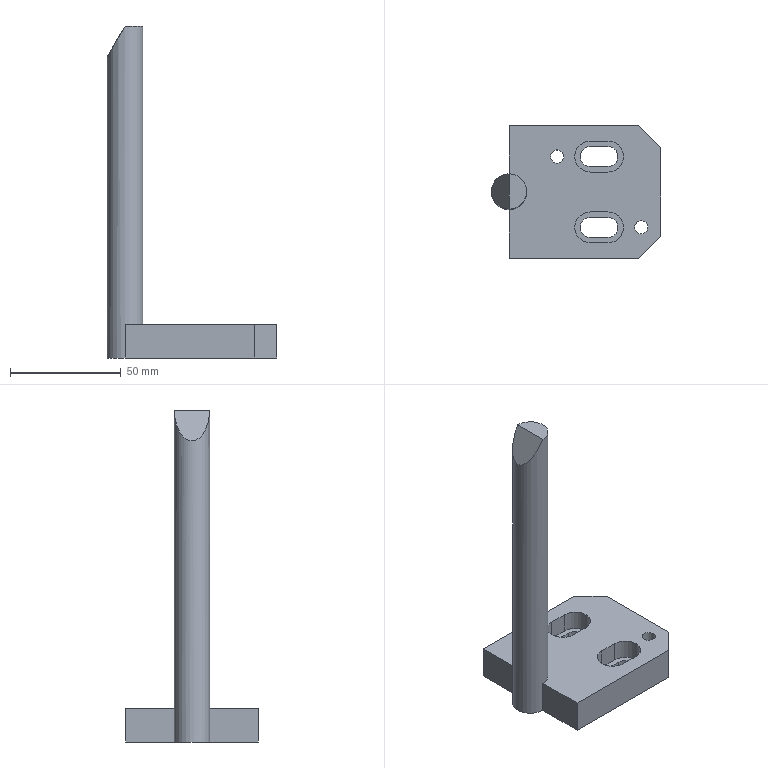Part | NX | features solid 2 | 1 solid | 32 faces | box 76.5 x 60 x 150 mm | volume 80948 mm3 | plane 21 | cylinder 11 | commonest cylinder face diameters 9 x4 14 x4 6 x2 16 x1
STEP:
#1=CARTESIAN_POINT('',(676.5,-352.,-140.));
#2=VERTEX_POINT('',#1);
#3=CARTESIAN_POINT('',(676.5,-352.,-125.));
#4=VERTEX_POINT('',#3);
#5=CARTESIAN_POINT('',(676.5,-352.,-140.));
#6=DIRECTION('',(0.,0.,1.));
#7=VECTOR('',#6,1000.);
#8=LINE('',#5,#7);
#9=EDGE_CURVE('',#2,#4,#8,.T.);
#10=ORIENTED_EDGE('',*,*,#9,.F.);
#11=CARTESIAN_POINT('',(676.5,-368.,-140.));
#12=VERTEX_POINT('',#11);
#13=CARTESIAN_POINT('',(676.5,-360.,-140.));
#14=DIRECTION('',(0.,0.,1.));
#15=DIRECTION('',(0.,1.,0.));
#16=AXIS2_PLACEMENT_3D('',#13,#14,#15);
#17=CIRCLE('',#16,8.);
#18=EDGE_CURVE('',#2,#12,#17,.T.);
#19=ORIENTED_EDGE('',*,*,#18,.T.);
#20=CARTESIAN_POINT('',(676.5,-368.,-125.));
#21=VERTEX_POINT('',#20);
#22=CARTESIAN_POINT('',(676.5,-368.,-140.));
#23=DIRECTION('',(0.,0.,1.));
#24=VECTOR('',#23,1000.);
#25=LINE('',#22,#24);
#26=EDGE_CURVE('',#21,#12,#25,.F.);
#27=ORIENTED_EDGE('',*,*,#26,.F.);
#28=CARTESIAN_POINT('',(676.5,-360.,-125.));
#29=DIRECTION('',(0.,0.,1.));
#30=DIRECTION('',(-1.,0.,0.));
#31=AXIS2_PLACEMENT_3D('',#28,#29,#30);
#32=CIRCLE('',#31,8.);
#33=EDGE_CURVE('',#21,#4,#32,.T.);
#34=ORIENTED_EDGE('',*,*,#33,.T.);
#35=EDGE_LOOP('',(#10,#19,#27,#34));
#36=FACE_BOUND('',#35,.T.);
#37=CARTESIAN_POINT('',(676.5,-368.,10.));
#38=VERTEX_POINT('',#37);
#39=CARTESIAN_POINT('',(676.5,-352.,10.));
#40=VERTEX_POINT('',#39);
#41=CARTESIAN_POINT('',(676.5,-360.,10.));
#42=DIRECTION('',(0.,0.,-1.));
#43=DIRECTION('',(-1.,0.,0.));
#44=AXIS2_PLACEMENT_3D('',#41,#42,#43);
#45=CIRCLE('',#44,8.);
#46=EDGE_CURVE('',#38,#40,#45,.F.);
#47=ORIENTED_EDGE('',*,*,#46,.F.);
#48=CARTESIAN_POINT('',(676.5,-360.,10.));
#49=DIRECTION('',(0.866,0.,-0.5));
#50=DIRECTION('',(0.5,0.,0.866));
#51=AXIS2_PLACEMENT_3D('',#48,#49,#50);
#52=ELLIPSE('',#51,16.,8.);
#53=EDGE_CURVE('',#40,#38,#52,.F.);
#54=ORIENTED_EDGE('',*,*,#53,.F.);
#55=EDGE_LOOP('',(#47,#54));
#56=FACE_BOUND('',#55,.T.);
#57=CARTESIAN_POINT('',(676.5,-360.,-140.));
#58=DIRECTION('',(0.,0.,1.));
#59=DIRECTION('',(-1.,0.,0.));
#60=AXIS2_PLACEMENT_3D('',#57,#58,#59);
#61=CYLINDRICAL_SURFACE('',#60,8.);
#62=ADVANCED_FACE('',(#36,#56),#61,.T.);
#63=ORIENTED_EDGE('',*,*,#46,.T.);
#64=CARTESIAN_POINT('',(676.5,-360.,10.));
#65=DIRECTION('',(0.,1.,0.));
#66=VECTOR('',#65,1000.);
#67=LINE('',#64,#66);
#68=EDGE_CURVE('',#38,#40,#67,.T.);
#69=ORIENTED_EDGE('',*,*,#68,.F.);
#70=EDGE_LOOP('',(#63,#69));
#71=FACE_BOUND('',#70,.T.);
#72=CARTESIAN_POINT('',(682.,-360.,10.));
#73=DIRECTION('',(0.,0.,1.));
#74=DIRECTION('',(-1.,0.,0.));
#75=AXIS2_PLACEMENT_3D('',#72,#73,#74);
#76=PLANE('',#75);
#77=ADVANCED_FACE('',(#71),#76,.T.);
#78=CARTESIAN_POINT('',(695.2,-344.,-125.));
#79=VERTEX_POINT('',#78);
#80=CARTESIAN_POINT('',(698.2,-344.,-125.));
#81=DIRECTION('',(0.,0.,1.));
#82=DIRECTION('',(-1.,0.,0.));
#83=AXIS2_PLACEMENT_3D('',#80,#81,#82);
#84=CIRCLE('',#83,3.);
#85=EDGE_CURVE('',#79,#79,#84,.F.);
#86=ORIENTED_EDGE('',*,*,#85,.T.);
#87=EDGE_LOOP('',(#86));
#88=FACE_BOUND('',#87,.T.);
#89=CARTESIAN_POINT('',(713.2,-351.,-125.));
#90=VERTEX_POINT('',#89);
#91=CARTESIAN_POINT('',(713.2,-337.,-125.));
#92=VERTEX_POINT('',#91);
#93=CARTESIAN_POINT('',(713.2,-344.,-125.));
#94=DIRECTION('',(0.,0.,1.));
#95=DIRECTION('',(-1.,0.,0.));
#96=AXIS2_PLACEMENT_3D('',#93,#94,#95);
#97=CIRCLE('',#96,7.);
#98=EDGE_CURVE('',#90,#92,#97,.F.);
#99=ORIENTED_EDGE('',*,*,#98,.T.);
#100=CARTESIAN_POINT('',(721.2,-337.,-125.));
#101=VERTEX_POINT('',#100);
#102=CARTESIAN_POINT('',(768.,-337.,-125.));
#103=DIRECTION('',(1.,0.,0.));
#104=VECTOR('',#103,1000.);
#105=LINE('',#102,#104);
#106=EDGE_CURVE('',#92,#101,#105,.T.);
#107=ORIENTED_EDGE('',*,*,#106,.T.);
#108=CARTESIAN_POINT('',(721.2,-351.,-125.));
#109=VERTEX_POINT('',#108);
#110=CARTESIAN_POINT('',(721.2,-344.,-125.));
#111=DIRECTION('',(0.,0.,1.));
#112=DIRECTION('',(-1.,0.,0.));
#113=AXIS2_PLACEMENT_3D('',#110,#111,#112);
#114=CIRCLE('',#113,7.);
#115=EDGE_CURVE('',#101,#109,#114,.F.);
#116=ORIENTED_EDGE('',*,*,#115,.T.);
#117=CARTESIAN_POINT('',(768.,-351.,-125.));
#118=DIRECTION('',(1.,0.,0.));
#119=VECTOR('',#118,1000.);
#120=LINE('',#117,#119);
#121=EDGE_CURVE('',#90,#109,#120,.T.);
#122=ORIENTED_EDGE('',*,*,#121,.F.);
#123=EDGE_LOOP('',(#99,#107,#116,#122));
#124=FACE_BOUND('',#123,.T.);
#125=CARTESIAN_POINT('',(733.2,-376.,-125.));
#126=VERTEX_POINT('',#125);
#127=CARTESIAN_POINT('',(736.2,-376.,-125.));
#128=DIRECTION('',(0.,0.,1.));
#129=DIRECTION('',(-1.,0.,0.));
#130=AXIS2_PLACEMENT_3D('',#127,#128,#129);
#131=CIRCLE('',#130,3.);
#132=EDGE_CURVE('',#126,#126,#131,.F.);
#133=ORIENTED_EDGE('',*,*,#132,.T.);
#134=EDGE_LOOP('',(#133));
#135=FACE_BOUND('',#134,.T.);
#136=CARTESIAN_POINT('',(713.2,-383.,-125.));
#137=VERTEX_POINT('',#136);
#138=CARTESIAN_POINT('',(721.2,-383.,-125.));
#139=VERTEX_POINT('',#138);
#140=CARTESIAN_POINT('',(713.2,-383.,-125.));
#141=DIRECTION('',(1.,0.,0.));
#142=VECTOR('',#141,1000.);
#143=LINE('',#140,#142);
#144=EDGE_CURVE('',#137,#139,#143,.T.);
#145=ORIENTED_EDGE('',*,*,#144,.F.);
#146=CARTESIAN_POINT('',(713.2,-369.,-125.));
#147=VERTEX_POINT('',#146);
#148=CARTESIAN_POINT('',(713.2,-376.,-125.));
#149=DIRECTION('',(0.,0.,1.));
#150=DIRECTION('',(-1.,0.,0.));
#151=AXIS2_PLACEMENT_3D('',#148,#149,#150);
#152=CIRCLE('',#151,7.);
#153=EDGE_CURVE('',#147,#137,#152,.T.);
#154=ORIENTED_EDGE('',*,*,#153,.F.);
#155=CARTESIAN_POINT('',(721.2,-369.,-125.));
#156=VERTEX_POINT('',#155);
#157=CARTESIAN_POINT('',(713.2,-369.,-125.));
#158=DIRECTION('',(1.,0.,0.));
#159=VECTOR('',#158,1000.);
#160=LINE('',#157,#159);
#161=EDGE_CURVE('',#147,#156,#160,.T.);
#162=ORIENTED_EDGE('',*,*,#161,.T.);
#163=CARTESIAN_POINT('',(721.2,-376.,-125.));
#164=DIRECTION('',(0.,0.,1.));
#165=DIRECTION('',(-1.,0.,0.));
#166=AXIS2_PLACEMENT_3D('',#163,#164,#165);
#167=CIRCLE('',#166,7.);
#168=EDGE_CURVE('',#139,#156,#167,.T.);
#169=ORIENTED_EDGE('',*,*,#168,.F.);
#170=EDGE_LOOP('',(#145,#154,#162,#169));
#171=FACE_BOUND('',#170,.T.);
#172=CARTESIAN_POINT('',(676.5,-390.,-125.));
#173=VERTEX_POINT('',#172);
#174=CARTESIAN_POINT('',(735.,-390.,-125.));
#175=VERTEX_POINT('',#174);
#176=CARTESIAN_POINT('',(688.,-390.,-125.));
#177=DIRECTION('',(1.,0.,0.));
#178=VECTOR('',#177,1000.);
#179=LINE('',#176,#178);
#180=EDGE_CURVE('',#173,#175,#179,.T.);
#181=ORIENTED_EDGE('',*,*,#180,.T.);
#182=CARTESIAN_POINT('',(745.,-380.,-125.));
#183=VERTEX_POINT('',#182);
#184=CARTESIAN_POINT('',(766.5,-358.5,-125.));
#185=DIRECTION('',(-0.7071,-0.7071,0.));
#186=VECTOR('',#185,1000.);
#187=LINE('',#184,#186);
#188=EDGE_CURVE('',#175,#183,#187,.F.);
#189=ORIENTED_EDGE('',*,*,#188,.T.);
#190=CARTESIAN_POINT('',(745.,-340.,-125.));
#191=VERTEX_POINT('',#190);
#192=CARTESIAN_POINT('',(745.,-360.,-125.));
#193=DIRECTION('',(0.,-1.,0.));
#194=VECTOR('',#193,1000.);
#195=LINE('',#192,#194);
#196=EDGE_CURVE('',#183,#191,#195,.F.);
#197=ORIENTED_EDGE('',*,*,#196,.T.);
#198=CARTESIAN_POINT('',(735.,-330.,-125.));
#199=VERTEX_POINT('',#198);
#200=CARTESIAN_POINT('',(766.5,-361.5,-125.));
#201=DIRECTION('',(-0.7071,0.7071,0.));
#202=VECTOR('',#201,1000.);
#203=LINE('',#200,#202);
#204=EDGE_CURVE('',#191,#199,#203,.T.);
#205=ORIENTED_EDGE('',*,*,#204,.T.);
#206=CARTESIAN_POINT('',(676.5,-330.,-125.));
#207=VERTEX_POINT('',#206);
#208=CARTESIAN_POINT('',(688.,-330.,-125.));
#209=DIRECTION('',(1.,0.,0.));
#210=VECTOR('',#209,1000.);
#211=LINE('',#208,#210);
#212=EDGE_CURVE('',#207,#199,#211,.T.);
#213=ORIENTED_EDGE('',*,*,#212,.F.);
#214=CARTESIAN_POINT('',(676.5,-330.,-125.));
#215=DIRECTION('',(0.,-1.,0.));
#216=VECTOR('',#215,1000.);
#217=LINE('',#214,#216);
#218=EDGE_CURVE('',#207,#4,#217,.T.);
#219=ORIENTED_EDGE('',*,*,#218,.T.);
#220=ORIENTED_EDGE('',*,*,#33,.F.);
#221=CARTESIAN_POINT('',(676.5,-330.,-125.));
#222=DIRECTION('',(0.,-1.,0.));
#223=VECTOR('',#222,1000.);
#224=LINE('',#221,#223);
#225=EDGE_CURVE('',#21,#173,#224,.T.);
#226=ORIENTED_EDGE('',*,*,#225,.T.);
#227=EDGE_LOOP('',(#181,#189,#197,#205,#213,#219,#220,#226));
#228=FACE_BOUND('',#227,.T.);
#229=CARTESIAN_POINT('',(768.,-360.,-125.));
#230=DIRECTION('',(0.,0.,1.));
#231=DIRECTION('',(-1.,0.,0.));
#232=AXIS2_PLACEMENT_3D('',#229,#230,#231);
#233=PLANE('',#232);
#234=ADVANCED_FACE('',(#88,#124,#135,#171,#228),#233,.T.);
#235=CARTESIAN_POINT('',(695.2,-344.,-140.));
#236=VERTEX_POINT('',#235);
#237=CARTESIAN_POINT('',(698.2,-344.,-140.));
#238=DIRECTION('',(0.,0.,1.));
#239=DIRECTION('',(-1.,0.,0.));
#240=AXIS2_PLACEMENT_3D('',#237,#238,#239);
#241=CIRCLE('',#240,3.);
#242=EDGE_CURVE('',#236,#236,#241,.T.);
#243=ORIENTED_EDGE('',*,*,#242,.T.);
#244=EDGE_LOOP('',(#243));
#245=FACE_BOUND('',#244,.T.);
#246=CARTESIAN_POINT('',(721.2,-380.5,-140.));
#247=VERTEX_POINT('',#246);
#248=CARTESIAN_POINT('',(721.2,-371.5,-140.));
#249=VERTEX_POINT('',#248);
#250=CARTESIAN_POINT('',(721.2,-376.,-140.));
#251=DIRECTION('',(0.,0.,1.));
#252=DIRECTION('',(-1.,0.,0.));
#253=AXIS2_PLACEMENT_3D('',#250,#251,#252);
#254=CIRCLE('',#253,4.5);
#255=EDGE_CURVE('',#247,#249,#254,.T.);
#256=ORIENTED_EDGE('',*,*,#255,.T.);
#257=CARTESIAN_POINT('',(713.2,-371.5,-140.));
#258=VERTEX_POINT('',#257);
#259=CARTESIAN_POINT('',(713.2,-371.5,-140.));
#260=DIRECTION('',(1.,0.,0.));
#261=VECTOR('',#260,1000.);
#262=LINE('',#259,#261);
#263=EDGE_CURVE('',#258,#249,#262,.T.);
#264=ORIENTED_EDGE('',*,*,#263,.F.);
#265=CARTESIAN_POINT('',(713.2,-380.5,-140.));
#266=VERTEX_POINT('',#265);
#267=CARTESIAN_POINT('',(713.2,-376.,-140.));
#268=DIRECTION('',(0.,0.,1.));
#269=DIRECTION('',(-1.,0.,0.));
#270=AXIS2_PLACEMENT_3D('',#267,#268,#269);
#271=CIRCLE('',#270,4.5);
#272=EDGE_CURVE('',#258,#266,#271,.T.);
#273=ORIENTED_EDGE('',*,*,#272,.T.);
#274=CARTESIAN_POINT('',(713.2,-380.5,-140.));
#275=DIRECTION('',(1.,0.,0.));
#276=VECTOR('',#275,1000.);
#277=LINE('',#274,#276);
#278=EDGE_CURVE('',#266,#247,#277,.T.);
#279=ORIENTED_EDGE('',*,*,#278,.T.);
#280=EDGE_LOOP('',(#256,#264,#273,#279));
#281=FACE_BOUND('',#280,.T.);
#282=CARTESIAN_POINT('',(733.2,-376.,-140.));
#283=VERTEX_POINT('',#282);
#284=CARTESIAN_POINT('',(736.2,-376.,-140.));
#285=DIRECTION('',(0.,0.,1.));
#286=DIRECTION('',(-1.,0.,0.));
#287=AXIS2_PLACEMENT_3D('',#284,#285,#286);
#288=CIRCLE('',#287,3.);
#289=EDGE_CURVE('',#283,#283,#288,.T.);
#290=ORIENTED_EDGE('',*,*,#289,.T.);
#291=EDGE_LOOP('',(#290));
#292=FACE_BOUND('',#291,.T.);
#293=CARTESIAN_POINT('',(721.2,-348.5,-140.));
#294=VERTEX_POINT('',#293);
#295=CARTESIAN_POINT('',(721.2,-339.5,-140.));
#296=VERTEX_POINT('',#295);
#297=CARTESIAN_POINT('',(721.2,-344.,-140.));
#298=DIRECTION('',(0.,0.,1.));
#299=DIRECTION('',(-1.,0.,0.));
#300=AXIS2_PLACEMENT_3D('',#297,#298,#299);
#301=CIRCLE('',#300,4.5);
#302=EDGE_CURVE('',#294,#296,#301,.T.);
#303=ORIENTED_EDGE('',*,*,#302,.T.);
#304=CARTESIAN_POINT('',(713.2,-339.5,-140.));
#305=VERTEX_POINT('',#304);
#306=CARTESIAN_POINT('',(723.2,-339.5,-140.));
#307=DIRECTION('',(-1.,0.,0.));
#308=VECTOR('',#307,1000.);
#309=LINE('',#306,#308);
#310=EDGE_CURVE('',#296,#305,#309,.T.);
#311=ORIENTED_EDGE('',*,*,#310,.T.);
#312=CARTESIAN_POINT('',(713.2,-348.5,-140.));
#313=VERTEX_POINT('',#312);
#314=CARTESIAN_POINT('',(713.2,-344.,-140.));
#315=DIRECTION('',(0.,0.,1.));
#316=DIRECTION('',(-1.,0.,0.));
#317=AXIS2_PLACEMENT_3D('',#314,#315,#316);
#318=CIRCLE('',#317,4.5);
#319=EDGE_CURVE('',#305,#313,#318,.T.);
#320=ORIENTED_EDGE('',*,*,#319,.T.);
#321=CARTESIAN_POINT('',(723.2,-348.5,-140.));
#322=DIRECTION('',(-1.,0.,0.));
#323=VECTOR('',#322,1000.);
#324=LINE('',#321,#323);
#325=EDGE_CURVE('',#294,#313,#324,.T.);
#326=ORIENTED_EDGE('',*,*,#325,.F.);
#327=EDGE_LOOP('',(#303,#311,#320,#326));
#328=FACE_BOUND('',#327,.T.);
#329=CARTESIAN_POINT('',(745.,-340.,-140.));
#330=VERTEX_POINT('',#329);
#331=CARTESIAN_POINT('',(745.,-380.,-140.));
#332=VERTEX_POINT('',#331);
#333=CARTESIAN_POINT('',(745.,-320.,-140.));
#334=DIRECTION('',(0.,1.,0.));
#335=VECTOR('',#334,1000.);
#336=LINE('',#333,#335);
#337=EDGE_CURVE('',#330,#332,#336,.F.);
#338=ORIENTED_EDGE('',*,*,#337,.T.);
#339=CARTESIAN_POINT('',(735.,-390.,-140.));
#340=VERTEX_POINT('',#339);
#341=CARTESIAN_POINT('',(745.,-380.,-140.));
#342=DIRECTION('',(0.7071,0.7071,0.));
#343=VECTOR('',#342,1000.);
#344=LINE('',#341,#343);
#345=EDGE_CURVE('',#332,#340,#344,.F.);
#346=ORIENTED_EDGE('',*,*,#345,.T.);
#347=CARTESIAN_POINT('',(676.5,-390.,-140.));
#348=VERTEX_POINT('',#347);
#349=CARTESIAN_POINT('',(688.,-390.,-140.));
#350=DIRECTION('',(1.,0.,0.));
#351=VECTOR('',#350,1000.);
#352=LINE('',#349,#351);
#353=EDGE_CURVE('',#348,#340,#352,.T.);
#354=ORIENTED_EDGE('',*,*,#353,.F.);
#355=CARTESIAN_POINT('',(676.5,-330.,-140.));
#356=DIRECTION('',(0.,-1.,0.));
#357=VECTOR('',#356,1000.);
#358=LINE('',#355,#357);
#359=EDGE_CURVE('',#12,#348,#358,.T.);
#360=ORIENTED_EDGE('',*,*,#359,.F.);
#361=ORIENTED_EDGE('',*,*,#18,.F.);
#362=CARTESIAN_POINT('',(676.5,-330.,-140.));
#363=VERTEX_POINT('',#362);
#364=CARTESIAN_POINT('',(676.5,-330.,-140.));
#365=DIRECTION('',(0.,-1.,0.));
#366=VECTOR('',#365,1000.);
#367=LINE('',#364,#366);
#368=EDGE_CURVE('',#363,#2,#367,.T.);
#369=ORIENTED_EDGE('',*,*,#368,.F.);
#370=CARTESIAN_POINT('',(735.,-330.,-140.));
#371=VERTEX_POINT('',#370);
#372=CARTESIAN_POINT('',(688.,-330.,-140.));
#373=DIRECTION('',(1.,0.,0.));
#374=VECTOR('',#373,1000.);
#375=LINE('',#372,#374);
#376=EDGE_CURVE('',#363,#371,#375,.T.);
#377=ORIENTED_EDGE('',*,*,#376,.T.);
#378=CARTESIAN_POINT('',(735.,-330.,-140.));
#379=DIRECTION('',(0.7071,-0.7071,0.));
#380=VECTOR('',#379,1000.);
#381=LINE('',#378,#380);
#382=EDGE_CURVE('',#371,#330,#381,.T.);
#383=ORIENTED_EDGE('',*,*,#382,.T.);
#384=EDGE_LOOP('',(#338,#346,#354,#360,#361,#369,#377,#383));
#385=FACE_BOUND('',#384,.T.);
#386=CARTESIAN_POINT('',(768.,-360.,-140.));
#387=DIRECTION('',(0.,0.,1.));
#388=DIRECTION('',(-1.,0.,0.));
#389=AXIS2_PLACEMENT_3D('',#386,#387,#388);
#390=PLANE('',#389);
#391=ADVANCED_FACE('',(#245,#281,#292,#328,#385),#390,.F.);
#392=ORIENTED_EDGE('',*,*,#212,.T.);
#393=CARTESIAN_POINT('',(735.,-330.,-125.));
#394=DIRECTION('',(0.,0.,-1.));
#395=VECTOR('',#394,1000.);
#396=LINE('',#393,#395);
#397=EDGE_CURVE('',#199,#371,#396,.T.);
#398=ORIENTED_EDGE('',*,*,#397,.T.);
#399=ORIENTED_EDGE('',*,*,#376,.F.);
#400=CARTESIAN_POINT('',(676.5,-330.,-125.));
#401=DIRECTION('',(0.,0.,-1.));
#402=VECTOR('',#401,1000.);
#403=LINE('',#400,#402);
#404=EDGE_CURVE('',#207,#363,#403,.T.);
#405=ORIENTED_EDGE('',*,*,#404,.F.);
#406=EDGE_LOOP('',(#392,#398,#399,#405));
#407=FACE_BOUND('',#406,.T.);
#408=CARTESIAN_POINT('',(688.,-330.,-125.));
#409=DIRECTION('',(0.,1.,0.));
#410=DIRECTION('',(0.,0.,-1.));
#411=AXIS2_PLACEMENT_3D('',#408,#409,#410);
#412=PLANE('',#411);
#413=ADVANCED_FACE('',(#407),#412,.T.);
#414=ORIENTED_EDGE('',*,*,#353,.T.);
#415=CARTESIAN_POINT('',(735.,-390.,-125.));
#416=DIRECTION('',(0.,0.,1.));
#417=VECTOR('',#416,1000.);
#418=LINE('',#415,#417);
#419=EDGE_CURVE('',#340,#175,#418,.T.);
#420=ORIENTED_EDGE('',*,*,#419,.T.);
#421=ORIENTED_EDGE('',*,*,#180,.F.);
#422=CARTESIAN_POINT('',(676.5,-390.,-125.));
#423=DIRECTION('',(0.,0.,-1.));
#424=VECTOR('',#423,1000.);
#425=LINE('',#422,#424);
#426=EDGE_CURVE('',#173,#348,#425,.T.);
#427=ORIENTED_EDGE('',*,*,#426,.T.);
#428=EDGE_LOOP('',(#414,#420,#421,#427));
#429=FACE_BOUND('',#428,.T.);
#430=CARTESIAN_POINT('',(688.,-390.,-125.));
#431=DIRECTION('',(0.,1.,0.));
#432=DIRECTION('',(-1.,0.,0.));
#433=AXIS2_PLACEMENT_3D('',#430,#431,#432);
#434=PLANE('',#433);
#435=ADVANCED_FACE('',(#429),#434,.F.);
#436=ORIENTED_EDGE('',*,*,#368,.T.);
#437=ORIENTED_EDGE('',*,*,#9,.T.);
#438=ORIENTED_EDGE('',*,*,#218,.F.);
#439=ORIENTED_EDGE('',*,*,#404,.T.);
#440=EDGE_LOOP('',(#436,#437,#438,#439));
#441=FACE_BOUND('',#440,.T.);
#442=CARTESIAN_POINT('',(676.5,-330.,-125.));
#443=DIRECTION('',(1.,0.,0.));
#444=DIRECTION('',(0.,0.,1.));
#445=AXIS2_PLACEMENT_3D('',#442,#443,#444);
#446=PLANE('',#445);
#447=ADVANCED_FACE('',(#441),#446,.F.);
#448=CARTESIAN_POINT('',(713.2,-371.5,-134.));
#449=VERTEX_POINT('',#448);
#450=CARTESIAN_POINT('',(721.2,-371.5,-134.));
#451=VERTEX_POINT('',#450);
#452=CARTESIAN_POINT('',(713.2,-371.5,-134.));
#453=DIRECTION('',(1.,0.,0.));
#454=VECTOR('',#453,1000.);
#455=LINE('',#452,#454);
#456=EDGE_CURVE('',#449,#451,#455,.T.);
#457=ORIENTED_EDGE('',*,*,#456,.F.);
#458=CARTESIAN_POINT('',(713.2,-371.5,-124.));
#459=DIRECTION('',(0.,0.,-1.));
#460=VECTOR('',#459,1000.);
#461=LINE('',#458,#460);
#462=EDGE_CURVE('',#449,#258,#461,.T.);
#463=ORIENTED_EDGE('',*,*,#462,.T.);
#464=ORIENTED_EDGE('',*,*,#263,.T.);
#465=CARTESIAN_POINT('',(721.2,-371.5,-124.));
#466=DIRECTION('',(0.,0.,-1.));
#467=VECTOR('',#466,1000.);
#468=LINE('',#465,#467);
#469=EDGE_CURVE('',#451,#249,#468,.T.);
#470=ORIENTED_EDGE('',*,*,#469,.F.);
#471=EDGE_LOOP('',(#457,#463,#464,#470));
#472=FACE_BOUND('',#471,.T.);
#473=CARTESIAN_POINT('',(713.2,-371.5,-124.));
#474=DIRECTION('',(0.,1.,0.));
#475=DIRECTION('',(0.,0.,-1.));
#476=AXIS2_PLACEMENT_3D('',#473,#474,#475);
#477=PLANE('',#476);
#478=ADVANCED_FACE('',(#472),#477,.F.);
#479=ORIENTED_EDGE('',*,*,#462,.F.);
#480=CARTESIAN_POINT('',(713.2,-380.5,-134.));
#481=VERTEX_POINT('',#480);
#482=CARTESIAN_POINT('',(713.2,-376.,-134.));
#483=DIRECTION('',(0.,0.,1.));
#484=DIRECTION('',(-1.,0.,0.));
#485=AXIS2_PLACEMENT_3D('',#482,#483,#484);
#486=CIRCLE('',#485,4.5);
#487=EDGE_CURVE('',#449,#481,#486,.T.);
#488=ORIENTED_EDGE('',*,*,#487,.T.);
#489=CARTESIAN_POINT('',(713.2,-380.5,-124.));
#490=DIRECTION('',(0.,0.,-1.));
#491=VECTOR('',#490,1000.);
#492=LINE('',#489,#491);
#493=EDGE_CURVE('',#481,#266,#492,.T.);
#494=ORIENTED_EDGE('',*,*,#493,.T.);
#495=ORIENTED_EDGE('',*,*,#272,.F.);
#496=EDGE_LOOP('',(#479,#488,#494,#495));
#497=FACE_BOUND('',#496,.T.);
#498=CARTESIAN_POINT('',(713.2,-376.,-124.));
#499=DIRECTION('',(0.,0.,-1.));
#500=DIRECTION('',(1.,0.,0.));
#501=AXIS2_PLACEMENT_3D('',#498,#499,#500);
#502=CYLINDRICAL_SURFACE('',#501,4.5);
#503=ADVANCED_FACE('',(#497),#502,.F.);
#504=ORIENTED_EDGE('',*,*,#493,.F.);
#505=CARTESIAN_POINT('',(721.2,-380.5,-134.));
#506=VERTEX_POINT('',#505);
#507=CARTESIAN_POINT('',(713.2,-380.5,-134.));
#508=DIRECTION('',(1.,0.,0.));
#509=VECTOR('',#508,1000.);
#510=LINE('',#507,#509);
#511=EDGE_CURVE('',#481,#506,#510,.T.);
#512=ORIENTED_EDGE('',*,*,#511,.T.);
#513=CARTESIAN_POINT('',(721.2,-380.5,-124.));
#514=DIRECTION('',(0.,0.,-1.));
#515=VECTOR('',#514,1000.);
#516=LINE('',#513,#515);
#517=EDGE_CURVE('',#506,#247,#516,.T.);
#518=ORIENTED_EDGE('',*,*,#517,.T.);
#519=ORIENTED_EDGE('',*,*,#278,.F.);
#520=EDGE_LOOP('',(#504,#512,#518,#519));
#521=FACE_BOUND('',#520,.T.);
#522=CARTESIAN_POINT('',(713.2,-380.5,-124.));
#523=DIRECTION('',(0.,1.,0.));
#524=DIRECTION('',(0.,0.,-1.));
#525=AXIS2_PLACEMENT_3D('',#522,#523,#524);
#526=PLANE('',#525);
#527=ADVANCED_FACE('',(#521),#526,.T.);
#528=ORIENTED_EDGE('',*,*,#517,.F.);
#529=CARTESIAN_POINT('',(721.2,-376.,-134.));
#530=DIRECTION('',(0.,0.,1.));
#531=DIRECTION('',(-1.,0.,0.));
#532=AXIS2_PLACEMENT_3D('',#529,#530,#531);
#533=CIRCLE('',#532,4.5);
#534=EDGE_CURVE('',#506,#451,#533,.T.);
#535=ORIENTED_EDGE('',*,*,#534,.T.);
#536=ORIENTED_EDGE('',*,*,#469,.T.);
#537=ORIENTED_EDGE('',*,*,#255,.F.);
#538=EDGE_LOOP('',(#528,#535,#536,#537));
#539=FACE_BOUND('',#538,.T.);
#540=CARTESIAN_POINT('',(721.2,-376.,-124.));
#541=DIRECTION('',(0.,0.,-1.));
#542=DIRECTION('',(1.,0.,0.));
#543=AXIS2_PLACEMENT_3D('',#540,#541,#542);
#544=CYLINDRICAL_SURFACE('',#543,4.5);
#545=ADVANCED_FACE('',(#539),#544,.F.);
#546=ORIENTED_EDGE('',*,*,#225,.F.);
#547=ORIENTED_EDGE('',*,*,#26,.T.);
#548=ORIENTED_EDGE('',*,*,#359,.T.);
#549=ORIENTED_EDGE('',*,*,#426,.F.);
#550=EDGE_LOOP('',(#546,#547,#548,#549));
#551=FACE_BOUND('',#550,.T.);
#552=CARTESIAN_POINT('',(676.5,-330.,-125.));
#553=DIRECTION('',(1.,0.,0.));
#554=DIRECTION('',(0.,0.,1.));
#555=AXIS2_PLACEMENT_3D('',#552,#553,#554);
#556=PLANE('',#555);
#557=ADVANCED_FACE('',(#551),#556,.F.);
#558=CARTESIAN_POINT('',(713.2,-337.,-134.));
#559=VERTEX_POINT('',#558);
#560=CARTESIAN_POINT('',(713.2,-337.,-124.));
#561=DIRECTION('',(0.,0.,-1.));
#562=VECTOR('',#561,1000.);
#563=LINE('',#560,#562);
#564=EDGE_CURVE('',#92,#559,#563,.T.);
#565=ORIENTED_EDGE('',*,*,#564,.T.);
#566=CARTESIAN_POINT('',(721.2,-337.,-134.));
#567=VERTEX_POINT('',#566);
#568=CARTESIAN_POINT('',(723.2,-337.,-134.));
#569=DIRECTION('',(-1.,0.,0.));
#570=VECTOR('',#569,1000.);
#571=LINE('',#568,#570);
#572=EDGE_CURVE('',#567,#559,#571,.T.);
#573=ORIENTED_EDGE('',*,*,#572,.F.);
#574=CARTESIAN_POINT('',(721.2,-337.,-124.));
#575=DIRECTION('',(0.,0.,-1.));
#576=VECTOR('',#575,1000.);
#577=LINE('',#574,#576);
#578=EDGE_CURVE('',#101,#567,#577,.T.);
#579=ORIENTED_EDGE('',*,*,#578,.F.);
#580=ORIENTED_EDGE('',*,*,#106,.F.);
#581=EDGE_LOOP('',(#565,#573,#579,#580));
#582=FACE_BOUND('',#581,.T.);
#583=CARTESIAN_POINT('',(723.2,-337.,-124.));
#584=DIRECTION('',(0.,-1.,0.));
#585=DIRECTION('',(0.,0.,1.));
#586=AXIS2_PLACEMENT_3D('',#583,#584,#585);
#587=PLANE('',#586);
#588=ADVANCED_FACE('',(#582),#587,.T.);
#589=CARTESIAN_POINT('',(713.2,-351.,-134.));
#590=VERTEX_POINT('',#589);
#591=CARTESIAN_POINT('',(713.2,-351.,-124.));
#592=DIRECTION('',(0.,0.,-1.));
#593=VECTOR('',#592,1000.);
#594=LINE('',#591,#593);
#595=EDGE_CURVE('',#90,#590,#594,.T.);
#596=ORIENTED_EDGE('',*,*,#595,.T.);
#597=CARTESIAN_POINT('',(713.2,-344.,-134.));
#598=DIRECTION('',(0.,0.,1.));
#599=DIRECTION('',(-1.,0.,0.));
#600=AXIS2_PLACEMENT_3D('',#597,#598,#599);
#601=CIRCLE('',#600,7.);
#602=EDGE_CURVE('',#559,#590,#601,.T.);
#603=ORIENTED_EDGE('',*,*,#602,.F.);
#604=ORIENTED_EDGE('',*,*,#564,.F.);
#605=ORIENTED_EDGE('',*,*,#98,.F.);
#606=EDGE_LOOP('',(#596,#603,#604,#605));
#607=FACE_BOUND('',#606,.T.);
#608=CARTESIAN_POINT('',(713.2,-344.,-124.));
#609=DIRECTION('',(0.,0.,-1.));
#610=DIRECTION('',(1.,0.,0.));
#611=AXIS2_PLACEMENT_3D('',#608,#609,#610);
#612=CYLINDRICAL_SURFACE('',#611,7.);
#613=ADVANCED_FACE('',(#607),#612,.F.);
#614=ORIENTED_EDGE('',*,*,#121,.T.);
#615=CARTESIAN_POINT('',(721.2,-351.,-134.));
#616=VERTEX_POINT('',#615);
#617=CARTESIAN_POINT('',(721.2,-351.,-124.));
#618=DIRECTION('',(0.,0.,-1.));
#619=VECTOR('',#618,1000.);
#620=LINE('',#617,#619);
#621=EDGE_CURVE('',#109,#616,#620,.T.);
#622=ORIENTED_EDGE('',*,*,#621,.T.);
#623=CARTESIAN_POINT('',(723.2,-351.,-134.));
#624=DIRECTION('',(-1.,0.,0.));
#625=VECTOR('',#624,1000.);
#626=LINE('',#623,#625);
#627=EDGE_CURVE('',#616,#590,#626,.T.);
#628=ORIENTED_EDGE('',*,*,#627,.T.);
#629=ORIENTED_EDGE('',*,*,#595,.F.);
#630=EDGE_LOOP('',(#614,#622,#628,#629));
#631=FACE_BOUND('',#630,.T.);
#632=CARTESIAN_POINT('',(723.2,-351.,-124.));
#633=DIRECTION('',(0.,-1.,0.));
#634=DIRECTION('',(0.,0.,1.));
#635=AXIS2_PLACEMENT_3D('',#632,#633,#634);
#636=PLANE('',#635);
#637=ADVANCED_FACE('',(#631),#636,.F.);
#638=ORIENTED_EDGE('',*,*,#578,.T.);
#639=CARTESIAN_POINT('',(721.2,-344.,-134.));
#640=DIRECTION('',(0.,0.,1.));
#641=DIRECTION('',(-1.,0.,0.));
#642=AXIS2_PLACEMENT_3D('',#639,#640,#641);
#643=CIRCLE('',#642,7.);
#644=EDGE_CURVE('',#616,#567,#643,.T.);
#645=ORIENTED_EDGE('',*,*,#644,.F.);
#646=ORIENTED_EDGE('',*,*,#621,.F.);
#647=ORIENTED_EDGE('',*,*,#115,.F.);
#648=EDGE_LOOP('',(#638,#645,#646,#647));
#649=FACE_BOUND('',#648,.T.);
#650=CARTESIAN_POINT('',(721.2,-344.,-124.));
#651=DIRECTION('',(0.,0.,-1.));
#652=DIRECTION('',(1.,0.,0.));
#653=AXIS2_PLACEMENT_3D('',#650,#651,#652);
#654=CYLINDRICAL_SURFACE('',#653,7.);
#655=ADVANCED_FACE('',(#649),#654,.F.);
#656=CARTESIAN_POINT('',(721.2,-339.5,-134.));
#657=VERTEX_POINT('',#656);
#658=CARTESIAN_POINT('',(713.2,-339.5,-134.));
#659=VERTEX_POINT('',#658);
#660=CARTESIAN_POINT('',(723.2,-339.5,-134.));
#661=DIRECTION('',(-1.,0.,0.));
#662=VECTOR('',#661,1000.);
#663=LINE('',#660,#662);
#664=EDGE_CURVE('',#657,#659,#663,.T.);
#665=ORIENTED_EDGE('',*,*,#664,.F.);
#666=CARTESIAN_POINT('',(721.2,-348.5,-134.));
#667=VERTEX_POINT('',#666);
#668=CARTESIAN_POINT('',(721.2,-344.,-134.));
#669=DIRECTION('',(0.,0.,1.));
#670=DIRECTION('',(-1.,0.,0.));
#671=AXIS2_PLACEMENT_3D('',#668,#669,#670);
#672=CIRCLE('',#671,4.5);
#673=EDGE_CURVE('',#667,#657,#672,.T.);
#674=ORIENTED_EDGE('',*,*,#673,.F.);
#675=CARTESIAN_POINT('',(713.2,-348.5,-134.));
#676=VERTEX_POINT('',#675);
#677=CARTESIAN_POINT('',(723.2,-348.5,-134.));
#678=DIRECTION('',(-1.,0.,0.));
#679=VECTOR('',#678,1000.);
#680=LINE('',#677,#679);
#681=EDGE_CURVE('',#667,#676,#680,.T.);
#682=ORIENTED_EDGE('',*,*,#681,.T.);
#683=CARTESIAN_POINT('',(713.2,-344.,-134.));
#684=DIRECTION('',(0.,0.,1.));
#685=DIRECTION('',(-1.,0.,0.));
#686=AXIS2_PLACEMENT_3D('',#683,#684,#685);
#687=CIRCLE('',#686,4.5);
#688=EDGE_CURVE('',#659,#676,#687,.T.);
#689=ORIENTED_EDGE('',*,*,#688,.F.);
#690=EDGE_LOOP('',(#665,#674,#682,#689));
#691=FACE_BOUND('',#690,.T.);
#692=ORIENTED_EDGE('',*,*,#572,.T.);
#693=ORIENTED_EDGE('',*,*,#602,.T.);
#694=ORIENTED_EDGE('',*,*,#627,.F.);
#695=ORIENTED_EDGE('',*,*,#644,.T.);
#696=EDGE_LOOP('',(#692,#693,#694,#695));
#697=FACE_BOUND('',#696,.T.);
#698=CARTESIAN_POINT('',(723.2,-344.,-134.));
#699=DIRECTION('',(0.,0.,1.));
#700=DIRECTION('',(-1.,0.,0.));
#701=AXIS2_PLACEMENT_3D('',#698,#699,#700);
#702=PLANE('',#701);
#703=ADVANCED_FACE('',(#691,#697),#702,.T.);
#704=ORIENTED_EDGE('',*,*,#132,.F.);
#705=EDGE_LOOP('',(#704));
#706=FACE_BOUND('',#705,.T.);
#707=ORIENTED_EDGE('',*,*,#289,.F.);
#708=EDGE_LOOP('',(#707));
#709=FACE_BOUND('',#708,.T.);
#710=CARTESIAN_POINT('',(736.2,-376.,-124.));
#711=DIRECTION('',(0.,0.,-1.));
#712=DIRECTION('',(1.,0.,0.));
#713=AXIS2_PLACEMENT_3D('',#710,#711,#712);
#714=CYLINDRICAL_SURFACE('',#713,3.);
#715=ADVANCED_FACE('',(#706,#709),#714,.F.);
#716=ORIENTED_EDGE('',*,*,#85,.F.);
#717=EDGE_LOOP('',(#716));
#718=FACE_BOUND('',#717,.T.);
#719=ORIENTED_EDGE('',*,*,#242,.F.);
#720=EDGE_LOOP('',(#719));
#721=FACE_BOUND('',#720,.T.);
#722=CARTESIAN_POINT('',(698.2,-344.,-124.));
#723=DIRECTION('',(0.,0.,-1.));
#724=DIRECTION('',(1.,0.,0.));
#725=AXIS2_PLACEMENT_3D('',#722,#723,#724);
#726=CYLINDRICAL_SURFACE('',#725,3.);
#727=ADVANCED_FACE('',(#718,#721),#726,.F.);
#728=CARTESIAN_POINT('',(713.2,-383.,-134.));
#729=VERTEX_POINT('',#728);
#730=CARTESIAN_POINT('',(721.2,-383.,-134.));
#731=VERTEX_POINT('',#730);
#732=CARTESIAN_POINT('',(713.2,-383.,-134.));
#733=DIRECTION('',(1.,0.,0.));
#734=VECTOR('',#733,1000.);
#735=LINE('',#732,#734);
#736=EDGE_CURVE('',#729,#731,#735,.T.);
#737=ORIENTED_EDGE('',*,*,#736,.T.);
#738=CARTESIAN_POINT('',(721.2,-369.,-134.));
#739=VERTEX_POINT('',#738);
#740=CARTESIAN_POINT('',(721.2,-376.,-134.));
#741=DIRECTION('',(0.,0.,1.));
#742=DIRECTION('',(-1.,0.,0.));
#743=AXIS2_PLACEMENT_3D('',#740,#741,#742);
#744=CIRCLE('',#743,7.);
#745=EDGE_CURVE('',#731,#739,#744,.T.);
#746=ORIENTED_EDGE('',*,*,#745,.T.);
#747=CARTESIAN_POINT('',(713.2,-369.,-134.));
#748=VERTEX_POINT('',#747);
#749=CARTESIAN_POINT('',(713.2,-369.,-134.));
#750=DIRECTION('',(1.,0.,0.));
#751=VECTOR('',#750,1000.);
#752=LINE('',#749,#751);
#753=EDGE_CURVE('',#748,#739,#752,.T.);
#754=ORIENTED_EDGE('',*,*,#753,.F.);
#755=CARTESIAN_POINT('',(713.2,-376.,-134.));
#756=DIRECTION('',(0.,0.,1.));
#757=DIRECTION('',(-1.,0.,0.));
#758=AXIS2_PLACEMENT_3D('',#755,#756,#757);
#759=CIRCLE('',#758,7.);
#760=EDGE_CURVE('',#748,#729,#759,.T.);
#761=ORIENTED_EDGE('',*,*,#760,.T.);
#762=EDGE_LOOP('',(#737,#746,#754,#761));
#763=FACE_BOUND('',#762,.T.);
#764=ORIENTED_EDGE('',*,*,#456,.T.);
#765=ORIENTED_EDGE('',*,*,#534,.F.);
#766=ORIENTED_EDGE('',*,*,#511,.F.);
#767=ORIENTED_EDGE('',*,*,#487,.F.);
#768=EDGE_LOOP('',(#764,#765,#766,#767));
#769=FACE_BOUND('',#768,.T.);
#770=CARTESIAN_POINT('',(723.2,-376.,-134.));
#771=DIRECTION('',(0.,0.,1.));
#772=DIRECTION('',(-1.,0.,0.));
#773=AXIS2_PLACEMENT_3D('',#770,#771,#772);
#774=PLANE('',#773);
#775=ADVANCED_FACE('',(#763,#769),#774,.T.);
#776=ORIENTED_EDGE('',*,*,#144,.T.);
#777=CARTESIAN_POINT('',(721.2,-383.,-134.));
#778=DIRECTION('',(0.,0.,1.));
#779=VECTOR('',#778,1000.);
#780=LINE('',#777,#779);
#781=EDGE_CURVE('',#731,#139,#780,.T.);
#782=ORIENTED_EDGE('',*,*,#781,.F.);
#783=ORIENTED_EDGE('',*,*,#736,.F.);
#784=CARTESIAN_POINT('',(713.2,-383.,-134.));
#785=DIRECTION('',(0.,0.,1.));
#786=VECTOR('',#785,1000.);
#787=LINE('',#784,#786);
#788=EDGE_CURVE('',#729,#137,#787,.T.);
#789=ORIENTED_EDGE('',*,*,#788,.T.);
#790=EDGE_LOOP('',(#776,#782,#783,#789));
#791=FACE_BOUND('',#790,.T.);
#792=CARTESIAN_POINT('',(713.2,-383.,-134.));
#793=DIRECTION('',(0.,-1.,0.));
#794=DIRECTION('',(0.,0.,1.));
#795=AXIS2_PLACEMENT_3D('',#792,#793,#794);
#796=PLANE('',#795);
#797=ADVANCED_FACE('',(#791),#796,.F.);
#798=ORIENTED_EDGE('',*,*,#168,.T.);
#799=CARTESIAN_POINT('',(721.2,-369.,-134.));
#800=DIRECTION('',(0.,0.,1.));
#801=VECTOR('',#800,1000.);
#802=LINE('',#799,#801);
#803=EDGE_CURVE('',#739,#156,#802,.T.);
#804=ORIENTED_EDGE('',*,*,#803,.F.);
#805=ORIENTED_EDGE('',*,*,#745,.F.);
#806=ORIENTED_EDGE('',*,*,#781,.T.);
#807=EDGE_LOOP('',(#798,#804,#805,#806));
#808=FACE_BOUND('',#807,.T.);
#809=CARTESIAN_POINT('',(721.2,-376.,-134.));
#810=DIRECTION('',(0.,0.,1.));
#811=DIRECTION('',(-1.,0.,0.));
#812=AXIS2_PLACEMENT_3D('',#809,#810,#811);
#813=CYLINDRICAL_SURFACE('',#812,7.);
#814=ADVANCED_FACE('',(#808),#813,.F.);
#815=ORIENTED_EDGE('',*,*,#161,.F.);
#816=CARTESIAN_POINT('',(713.2,-369.,-134.));
#817=DIRECTION('',(0.,0.,1.));
#818=VECTOR('',#817,1000.);
#819=LINE('',#816,#818);
#820=EDGE_CURVE('',#748,#147,#819,.T.);
#821=ORIENTED_EDGE('',*,*,#820,.F.);
#822=ORIENTED_EDGE('',*,*,#753,.T.);
#823=ORIENTED_EDGE('',*,*,#803,.T.);
#824=EDGE_LOOP('',(#815,#821,#822,#823));
#825=FACE_BOUND('',#824,.T.);
#826=CARTESIAN_POINT('',(713.2,-369.,-134.));
#827=DIRECTION('',(0.,-1.,0.));
#828=DIRECTION('',(0.,0.,1.));
#829=AXIS2_PLACEMENT_3D('',#826,#827,#828);
#830=PLANE('',#829);
#831=ADVANCED_FACE('',(#825),#830,.T.);
#832=ORIENTED_EDGE('',*,*,#153,.T.);
#833=ORIENTED_EDGE('',*,*,#788,.F.);
#834=ORIENTED_EDGE('',*,*,#760,.F.);
#835=ORIENTED_EDGE('',*,*,#820,.T.);
#836=EDGE_LOOP('',(#832,#833,#834,#835));
#837=FACE_BOUND('',#836,.T.);
#838=CARTESIAN_POINT('',(713.2,-376.,-134.));
#839=DIRECTION('',(0.,0.,1.));
#840=DIRECTION('',(-1.,0.,0.));
#841=AXIS2_PLACEMENT_3D('',#838,#839,#840);
#842=CYLINDRICAL_SURFACE('',#841,7.);
#843=ADVANCED_FACE('',(#837),#842,.F.);
#844=ORIENTED_EDGE('',*,*,#664,.T.);
#845=CARTESIAN_POINT('',(713.2,-339.5,-140.));
#846=DIRECTION('',(0.,0.,1.));
#847=VECTOR('',#846,1000.);
#848=LINE('',#845,#847);
#849=EDGE_CURVE('',#305,#659,#848,.T.);
#850=ORIENTED_EDGE('',*,*,#849,.F.);
#851=ORIENTED_EDGE('',*,*,#310,.F.);
#852=CARTESIAN_POINT('',(721.2,-339.5,-140.));
#853=DIRECTION('',(0.,0.,1.));
#854=VECTOR('',#853,1000.);
#855=LINE('',#852,#854);
#856=EDGE_CURVE('',#296,#657,#855,.T.);
#857=ORIENTED_EDGE('',*,*,#856,.T.);
#858=EDGE_LOOP('',(#844,#850,#851,#857));
#859=FACE_BOUND('',#858,.T.);
#860=CARTESIAN_POINT('',(723.2,-339.5,-140.));
#861=DIRECTION('',(0.,1.,0.));
#862=DIRECTION('',(0.,0.,-1.));
#863=AXIS2_PLACEMENT_3D('',#860,#861,#862);
#864=PLANE('',#863);
#865=ADVANCED_FACE('',(#859),#864,.F.);
#866=ORIENTED_EDGE('',*,*,#688,.T.);
#867=CARTESIAN_POINT('',(713.2,-348.5,-140.));
#868=DIRECTION('',(0.,0.,1.));
#869=VECTOR('',#868,1000.);
#870=LINE('',#867,#869);
#871=EDGE_CURVE('',#313,#676,#870,.T.);
#872=ORIENTED_EDGE('',*,*,#871,.F.);
#873=ORIENTED_EDGE('',*,*,#319,.F.);
#874=ORIENTED_EDGE('',*,*,#849,.T.);
#875=EDGE_LOOP('',(#866,#872,#873,#874));
#876=FACE_BOUND('',#875,.T.);
#877=CARTESIAN_POINT('',(713.2,-344.,-140.));
#878=DIRECTION('',(0.,0.,1.));
#879=DIRECTION('',(-1.,0.,0.));
#880=AXIS2_PLACEMENT_3D('',#877,#878,#879);
#881=CYLINDRICAL_SURFACE('',#880,4.5);
#882=ADVANCED_FACE('',(#876),#881,.F.);
#883=ORIENTED_EDGE('',*,*,#681,.F.);
#884=CARTESIAN_POINT('',(721.2,-348.5,-140.));
#885=DIRECTION('',(0.,0.,1.));
#886=VECTOR('',#885,1000.);
#887=LINE('',#884,#886);
#888=EDGE_CURVE('',#294,#667,#887,.T.);
#889=ORIENTED_EDGE('',*,*,#888,.F.);
#890=ORIENTED_EDGE('',*,*,#325,.T.);
#891=ORIENTED_EDGE('',*,*,#871,.T.);
#892=EDGE_LOOP('',(#883,#889,#890,#891));
#893=FACE_BOUND('',#892,.T.);
#894=CARTESIAN_POINT('',(723.2,-348.5,-140.));
#895=DIRECTION('',(0.,1.,0.));
#896=DIRECTION('',(0.,0.,-1.));
#897=AXIS2_PLACEMENT_3D('',#894,#895,#896);
#898=PLANE('',#897);
#899=ADVANCED_FACE('',(#893),#898,.T.);
#900=ORIENTED_EDGE('',*,*,#673,.T.);
#901=ORIENTED_EDGE('',*,*,#856,.F.);
#902=ORIENTED_EDGE('',*,*,#302,.F.);
#903=ORIENTED_EDGE('',*,*,#888,.T.);
#904=EDGE_LOOP('',(#900,#901,#902,#903));
#905=FACE_BOUND('',#904,.T.);
#906=CARTESIAN_POINT('',(721.2,-344.,-140.));
#907=DIRECTION('',(0.,0.,1.));
#908=DIRECTION('',(-1.,0.,0.));
#909=AXIS2_PLACEMENT_3D('',#906,#907,#908);
#910=CYLINDRICAL_SURFACE('',#909,4.5);
#911=ADVANCED_FACE('',(#905),#910,.F.);
#912=ORIENTED_EDGE('',*,*,#196,.F.);
#913=CARTESIAN_POINT('',(745.,-380.,-140.));
#914=DIRECTION('',(0.,0.,1.));
#915=VECTOR('',#914,1000.);
#916=LINE('',#913,#915);
#917=EDGE_CURVE('',#183,#332,#916,.F.);
#918=ORIENTED_EDGE('',*,*,#917,.T.);
#919=ORIENTED_EDGE('',*,*,#337,.F.);
#920=CARTESIAN_POINT('',(745.,-340.,-140.));
#921=DIRECTION('',(0.,0.,-1.));
#922=VECTOR('',#921,1000.);
#923=LINE('',#920,#922);
#924=EDGE_CURVE('',#330,#191,#923,.F.);
#925=ORIENTED_EDGE('',*,*,#924,.T.);
#926=EDGE_LOOP('',(#912,#918,#919,#925));
#927=FACE_BOUND('',#926,.T.);
#928=CARTESIAN_POINT('',(745.,-320.,-140.));
#929=DIRECTION('',(-1.,0.,0.));
#930=DIRECTION('',(0.,-1.,0.));
#931=AXIS2_PLACEMENT_3D('',#928,#929,#930);
#932=PLANE('',#931);
#933=ADVANCED_FACE('',(#927),#932,.F.);
#934=ORIENTED_EDGE('',*,*,#204,.F.);
#935=ORIENTED_EDGE('',*,*,#924,.F.);
#936=ORIENTED_EDGE('',*,*,#382,.F.);
#937=ORIENTED_EDGE('',*,*,#397,.F.);
#938=EDGE_LOOP('',(#934,#935,#936,#937));
#939=FACE_BOUND('',#938,.T.);
#940=CARTESIAN_POINT('',(735.,-330.,-125.));
#941=DIRECTION('',(0.7071,0.7071,0.));
#942=DIRECTION('',(-0.7071,0.7071,0.));
#943=AXIS2_PLACEMENT_3D('',#940,#941,#942);
#944=PLANE('',#943);
#945=ADVANCED_FACE('',(#939),#944,.T.);
#946=ORIENTED_EDGE('',*,*,#188,.F.);
#947=ORIENTED_EDGE('',*,*,#419,.F.);
#948=ORIENTED_EDGE('',*,*,#345,.F.);
#949=ORIENTED_EDGE('',*,*,#917,.F.);
#950=EDGE_LOOP('',(#946,#947,#948,#949));
#951=FACE_BOUND('',#950,.T.);
#952=CARTESIAN_POINT('',(745.,-380.,-140.));
#953=DIRECTION('',(-0.7071,0.7071,0.));
#954=DIRECTION('',(-0.7071,-0.7071,0.));
#955=AXIS2_PLACEMENT_3D('',#952,#953,#954);
#956=PLANE('',#955);
#957=ADVANCED_FACE('',(#951),#956,.F.);
#958=ORIENTED_EDGE('',*,*,#53,.T.);
#959=ORIENTED_EDGE('',*,*,#68,.T.);
#960=EDGE_LOOP('',(#958,#959));
#961=FACE_BOUND('',#960,.T.);
#962=CARTESIAN_POINT('',(701.5,-352.,53.301));
#963=DIRECTION('',(-0.866,0.,0.5));
#964=DIRECTION('',(-0.5,0.,-0.866));
#965=AXIS2_PLACEMENT_3D('',#962,#963,#964);
#966=PLANE('',#965);
#967=ADVANCED_FACE('',(#961),#966,.T.);
#968=CLOSED_SHELL('',(#62,#77,#234,#391,#413,#435,#447,#478,#503,#527,#545,#557,#588,#613,#637,#655,#703,#715,#727,#775,#797,#814,#831,#843,#865,#882,#899,#911,#933,#945,#957,#967));
#969=MANIFOLD_SOLID_BREP('',#968);
#970=(LENGTH_UNIT()NAMED_UNIT(*)SI_UNIT(.MILLI.,.METRE.));
#971=UNCERTAINTY_MEASURE_WITH_UNIT(LENGTH_MEASURE(0.00001),#970,'','');
#972=(NAMED_UNIT(*)PLANE_ANGLE_UNIT()SI_UNIT($,.RADIAN.));
#973=(NAMED_UNIT(*)SI_UNIT($,.STERADIAN.)SOLID_ANGLE_UNIT());
#974=(GEOMETRIC_REPRESENTATION_CONTEXT(3)GLOBAL_UNCERTAINTY_ASSIGNED_CONTEXT((#971))GLOBAL_UNIT_ASSIGNED_CONTEXT((#970,#972,#973))REPRESENTATION_CONTEXT('',''));
#975=ADVANCED_BREP_SHAPE_REPRESENTATION('',(#969),#974);